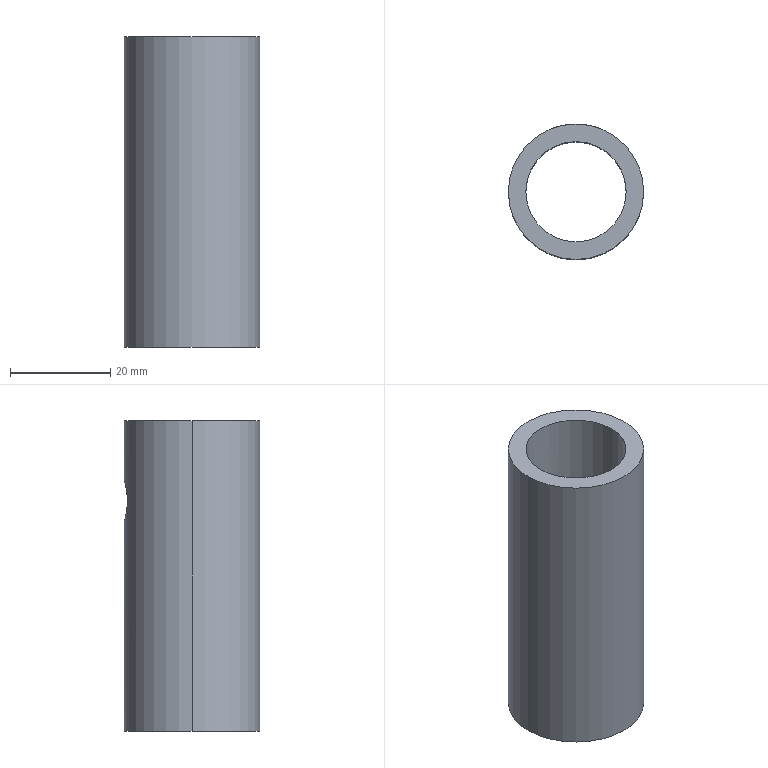Part | SolidWorks | features Extrusion 1, ICE 1 | 1 solid | 8 faces | box 27 x 27 x 62 mm | volume 15842 mm3 | cylinder 6 | plane 2 | commonest cylinder face diameters 8 x2 20 x2 27 x2
STEP:
#1=CARTESIAN_POINT('',(0.,13.5,-12.));
#2=VERTEX_POINT('',#1);
#3=CARTESIAN_POINT('',(0.,13.5,-20.));
#4=VERTEX_POINT('',#3);
#5=CARTESIAN_POINT('',(0.,13.5,-12.));
#6=CARTESIAN_POINT('',(-0.2619,13.5,-12.));
#7=CARTESIAN_POINT('',(-0.5246,13.492,-12.026));
#8=CARTESIAN_POINT('',(-1.044,13.462,-12.13));
#9=CARTESIAN_POINT('',(-1.294,13.44,-12.206));
#10=CARTESIAN_POINT('',(-1.776,13.385,-12.406));
#11=CARTESIAN_POINT('',(-2.01,13.351,-12.532));
#12=CARTESIAN_POINT('',(-2.443,13.279,-12.822));
#13=CARTESIAN_POINT('',(-2.643,13.24,-12.987));
#14=CARTESIAN_POINT('',(-3.013,13.161,-13.356));
#15=CARTESIAN_POINT('',(-3.18,13.121,-13.559));
#16=CARTESIAN_POINT('',(-3.468,13.048,-13.99));
#17=CARTESIAN_POINT('',(-3.592,13.014,-14.22));
#18=CARTESIAN_POINT('',(-3.795,12.956,-14.708));
#19=CARTESIAN_POINT('',(-3.871,12.933,-14.958));
#20=CARTESIAN_POINT('',(-3.973,12.902,-15.47));
#21=CARTESIAN_POINT('',(-4.,12.894,-15.736));
#22=CARTESIAN_POINT('',(-4.,12.894,-16.263));
#23=CARTESIAN_POINT('',(-3.974,12.902,-16.524));
#24=CARTESIAN_POINT('',(-3.872,12.933,-17.039));
#25=CARTESIAN_POINT('',(-3.794,12.956,-17.294));
#26=CARTESIAN_POINT('',(-3.594,13.013,-17.776));
#27=CARTESIAN_POINT('',(-3.471,13.047,-18.006));
#28=CARTESIAN_POINT('',(-3.178,13.121,-18.443));
#29=CARTESIAN_POINT('',(-3.013,13.161,-18.644));
#30=CARTESIAN_POINT('',(-2.646,13.239,-19.011));
#31=CARTESIAN_POINT('',(-2.442,13.279,-19.178));
#32=CARTESIAN_POINT('',(-2.009,13.352,-19.469));
#33=CARTESIAN_POINT('',(-1.78,13.384,-19.592));
#34=CARTESIAN_POINT('',(-1.297,13.44,-19.793));
#35=CARTESIAN_POINT('',(-1.042,13.462,-19.871));
#36=CARTESIAN_POINT('',(-0.5274,13.492,-19.974));
#37=CARTESIAN_POINT('',(-0.2658,13.5,-20.));
#38=CARTESIAN_POINT('',(0.,13.5,-20.));
#39=B_SPLINE_CURVE_WITH_KNOTS('',3,(#5,#6,#7,#8,#9,#10,#11,#12,#13,#14,#15,#16,#17,#18,#19,#20,#21,#22,#23,#24,#25,#26,#27,#28,#29,#30,#31,#32,#33,#34,#35,#36,#37,#38),.UNSPECIFIED.,.F.,.F.,(4,2,2,2,2,2,2,2,2,2,2,2,2,2,2,2,4),(0.01258,0.01336,0.01415,0.01493,0.01572,0.01651,0.01729,0.01808,0.01886,0.01965,0.02044,0.02122,0.02201,0.02279,0.02358,0.02436,0.02515),.UNSPECIFIED.);
#40=EDGE_CURVE('',#2,#4,#39,.T.);
#41=ORIENTED_EDGE('',*,*,#40,.F.);
#42=CARTESIAN_POINT('',(0.,10.,-12.));
#43=VERTEX_POINT('',#42);
#44=CARTESIAN_POINT('',(0.,62.,-12.));
#45=DIRECTION('',(0.,-1.,0.));
#46=VECTOR('',#45,1000.);
#47=LINE('',#44,#46);
#48=EDGE_CURVE('',#2,#43,#47,.T.);
#49=ORIENTED_EDGE('',*,*,#48,.T.);
#50=CARTESIAN_POINT('',(0.,10.,-20.));
#51=VERTEX_POINT('',#50);
#52=CARTESIAN_POINT('',(0.,10.,-12.));
#53=CARTESIAN_POINT('',(-0.2631,10.,-12.));
#54=CARTESIAN_POINT('',(-0.5298,9.989,-12.026));
#55=CARTESIAN_POINT('',(-1.048,9.948,-12.131));
#56=CARTESIAN_POINT('',(-1.299,9.918,-12.208));
#57=CARTESIAN_POINT('',(-1.782,9.843,-12.409));
#58=CARTESIAN_POINT('',(-2.015,9.797,-12.535));
#59=CARTESIAN_POINT('',(-2.446,9.699,-12.824));
#60=CARTESIAN_POINT('',(-2.646,9.645,-12.989));
#61=CARTESIAN_POINT('',(-3.015,9.537,-13.358));
#62=CARTESIAN_POINT('',(-3.179,9.483,-13.558));
#63=CARTESIAN_POINT('',(-3.466,9.381,-13.987));
#64=CARTESIAN_POINT('',(-3.592,9.333,-14.22));
#65=CARTESIAN_POINT('',(-3.793,9.253,-14.703));
#66=CARTESIAN_POINT('',(-3.869,9.221,-14.952));
#67=CARTESIAN_POINT('',(-3.973,9.177,-15.468));
#68=CARTESIAN_POINT('',(-4.,9.165,-15.736));
#69=CARTESIAN_POINT('',(-4.,9.165,-16.263));
#70=CARTESIAN_POINT('',(-3.974,9.177,-16.525));
#71=CARTESIAN_POINT('',(-3.87,9.221,-17.046));
#72=CARTESIAN_POINT('',(-3.792,9.254,-17.298));
#73=CARTESIAN_POINT('',(-3.592,9.333,-17.78));
#74=CARTESIAN_POINT('',(-3.467,9.381,-18.013));
#75=CARTESIAN_POINT('',(-3.177,9.483,-18.444));
#76=CARTESIAN_POINT('',(-3.013,9.537,-18.644));
#77=CARTESIAN_POINT('',(-2.646,9.645,-19.011));
#78=CARTESIAN_POINT('',(-2.443,9.699,-19.178));
#79=CARTESIAN_POINT('',(-2.014,9.798,-19.466));
#80=CARTESIAN_POINT('',(-1.785,9.842,-19.589));
#81=CARTESIAN_POINT('',(-1.298,9.918,-19.793));
#82=CARTESIAN_POINT('',(-1.046,9.948,-19.87));
#83=CARTESIAN_POINT('',(-0.5323,9.989,-19.973));
#84=CARTESIAN_POINT('',(-0.2671,10.,-20.));
#85=CARTESIAN_POINT('',(0.,10.,-20.));
#86=B_SPLINE_CURVE_WITH_KNOTS('',3,(#52,#53,#54,#55,#56,#57,#58,#59,#60,#61,#62,#63,#64,#65,#66,#67,#68,#69,#70,#71,#72,#73,#74,#75,#76,#77,#78,#79,#80,#81,#82,#83,#84,#85),.UNSPECIFIED.,.F.,.F.,(4,2,2,2,2,2,2,2,2,2,2,2,2,2,2,2,4),(0.01264,0.01343,0.01422,0.01501,0.0158,0.01659,0.01738,0.01817,0.01896,0.01974,0.02053,0.02132,0.02211,0.0229,0.02369,0.02448,0.02527),.UNSPECIFIED.);
#87=EDGE_CURVE('',#43,#51,#86,.T.);
#88=ORIENTED_EDGE('',*,*,#87,.T.);
#89=CARTESIAN_POINT('',(0.,62.,-20.));
#90=DIRECTION('',(0.,-1.,0.));
#91=VECTOR('',#90,1000.);
#92=LINE('',#89,#91);
#93=EDGE_CURVE('',#4,#51,#92,.T.);
#94=ORIENTED_EDGE('',*,*,#93,.F.);
#95=EDGE_LOOP('',(#41,#49,#88,#94));
#96=FACE_OUTER_BOUND('',#95,.T.);
#97=CARTESIAN_POINT('',(0.,62.,-16.));
#98=DIRECTION('',(0.,-1.,0.));
#99=DIRECTION('',(0.,0.,-1.));
#100=AXIS2_PLACEMENT_3D('',#97,#98,#99);
#101=CYLINDRICAL_SURFACE('',#100,4.);
#102=ADVANCED_FACE('',(#96),#101,.F.);
#103=CARTESIAN_POINT('',(-10.,0.,-62.));
#104=VERTEX_POINT('',#103);
#105=CARTESIAN_POINT('',(10.,0.,-62.));
#106=VERTEX_POINT('',#105);
#107=CARTESIAN_POINT('',(0.,0.,-62.));
#108=DIRECTION('',(0.,0.,1.));
#109=DIRECTION('',(1.,0.,0.));
#110=AXIS2_PLACEMENT_3D('',#107,#108,#109);
#111=CIRCLE('',#110,10.);
#112=EDGE_CURVE('',#104,#106,#111,.T.);
#113=ORIENTED_EDGE('',*,*,#112,.F.);
#114=CARTESIAN_POINT('',(-10.,0.,0.));
#115=VERTEX_POINT('',#114);
#116=CARTESIAN_POINT('',(-10.,0.,-62.));
#117=DIRECTION('',(0.,0.,1.));
#118=VECTOR('',#117,1000.);
#119=LINE('',#116,#118);
#120=EDGE_CURVE('',#104,#115,#119,.T.);
#121=ORIENTED_EDGE('',*,*,#120,.T.);
#122=CARTESIAN_POINT('',(10.,0.,0.));
#123=VERTEX_POINT('',#122);
#124=CARTESIAN_POINT('',(0.,0.,0.));
#125=DIRECTION('',(0.,0.,1.));
#126=DIRECTION('',(1.,0.,0.));
#127=AXIS2_PLACEMENT_3D('',#124,#125,#126);
#128=CIRCLE('',#127,10.);
#129=EDGE_CURVE('',#115,#123,#128,.T.);
#130=ORIENTED_EDGE('',*,*,#129,.T.);
#131=CARTESIAN_POINT('',(10.,0.,-62.));
#132=DIRECTION('',(0.,0.,1.));
#133=VECTOR('',#132,1000.);
#134=LINE('',#131,#133);
#135=EDGE_CURVE('',#106,#123,#134,.T.);
#136=ORIENTED_EDGE('',*,*,#135,.F.);
#137=EDGE_LOOP('',(#113,#121,#130,#136));
#138=FACE_OUTER_BOUND('',#137,.T.);
#139=CARTESIAN_POINT('',(0.,0.,-62.));
#140=DIRECTION('',(0.,0.,1.));
#141=DIRECTION('',(1.,0.,0.));
#142=AXIS2_PLACEMENT_3D('',#139,#140,#141);
#143=CYLINDRICAL_SURFACE('',#142,10.);
#144=ADVANCED_FACE('',(#138),#143,.F.);
#145=CARTESIAN_POINT('',(0.,13.5,-20.));
#146=CARTESIAN_POINT('',(0.2659,13.5,-20.));
#147=CARTESIAN_POINT('',(0.5271,13.492,-19.974));
#148=CARTESIAN_POINT('',(1.04,13.462,-19.871));
#149=CARTESIAN_POINT('',(1.295,13.44,-19.794));
#150=CARTESIAN_POINT('',(1.779,13.384,-19.592));
#151=CARTESIAN_POINT('',(2.008,13.352,-19.469));
#152=CARTESIAN_POINT('',(2.442,13.279,-19.179));
#153=CARTESIAN_POINT('',(2.646,13.239,-19.011));
#154=CARTESIAN_POINT('',(3.013,13.161,-18.644));
#155=CARTESIAN_POINT('',(3.178,13.122,-18.443));
#156=CARTESIAN_POINT('',(3.47,13.047,-18.007));
#157=CARTESIAN_POINT('',(3.593,13.013,-17.776));
#158=CARTESIAN_POINT('',(3.793,12.957,-17.296));
#159=CARTESIAN_POINT('',(3.871,12.933,-17.042));
#160=CARTESIAN_POINT('',(3.974,12.902,-16.525));
#161=CARTESIAN_POINT('',(4.,12.894,-16.264));
#162=CARTESIAN_POINT('',(4.,12.894,-15.739));
#163=CARTESIAN_POINT('',(3.974,12.902,-15.472));
#164=CARTESIAN_POINT('',(3.871,12.933,-14.958));
#165=CARTESIAN_POINT('',(3.795,12.956,-14.708));
#166=CARTESIAN_POINT('',(3.593,13.014,-14.222));
#167=CARTESIAN_POINT('',(3.468,13.048,-13.99));
#168=CARTESIAN_POINT('',(3.179,13.121,-13.559));
#169=CARTESIAN_POINT('',(3.012,13.161,-13.355));
#170=CARTESIAN_POINT('',(2.643,13.24,-12.986));
#171=CARTESIAN_POINT('',(2.442,13.279,-12.822));
#172=CARTESIAN_POINT('',(2.01,13.351,-12.532));
#173=CARTESIAN_POINT('',(1.776,13.385,-12.406));
#174=CARTESIAN_POINT('',(1.294,13.44,-12.206));
#175=CARTESIAN_POINT('',(1.044,13.462,-12.13));
#176=CARTESIAN_POINT('',(0.5275,13.492,-12.026));
#177=CARTESIAN_POINT('',(0.262,13.5,-12.));
#178=CARTESIAN_POINT('',(0.,13.5,-12.));
#179=B_SPLINE_CURVE_WITH_KNOTS('',3,(#145,#146,#147,#148,#149,#150,#151,#152,#153,#154,#155,#156,#157,#158,#159,#160,#161,#162,#163,#164,#165,#166,#167,#168,#169,#170,#171,#172,#173,#174,#175,#176,#177,#178),.UNSPECIFIED.,.F.,.F.,(4,2,2,2,2,2,2,2,2,2,2,2,2,2,2,2,4),(0.,0.0007861,0.001572,0.002358,0.003144,0.00393,0.004716,0.005502,0.006288,0.007074,0.007861,0.008647,0.009433,0.01022,0.011,0.01179,0.01258),.UNSPECIFIED.);
#180=EDGE_CURVE('',#4,#2,#179,.T.);
#181=ORIENTED_EDGE('',*,*,#180,.T.);
#182=ORIENTED_EDGE('',*,*,#40,.T.);
#183=EDGE_LOOP('',(#181,#182));
#184=FACE_BOUND('',#183,.T.);
#185=CARTESIAN_POINT('',(13.5,0.,-62.));
#186=VERTEX_POINT('',#185);
#187=CARTESIAN_POINT('',(-13.5,0.,-62.));
#188=VERTEX_POINT('',#187);
#189=CARTESIAN_POINT('',(0.,0.,-62.));
#190=DIRECTION('',(0.,0.,1.));
#191=DIRECTION('',(1.,0.,0.));
#192=AXIS2_PLACEMENT_3D('',#189,#190,#191);
#193=CIRCLE('',#192,13.5);
#194=EDGE_CURVE('',#186,#188,#193,.T.);
#195=ORIENTED_EDGE('',*,*,#194,.T.);
#196=CARTESIAN_POINT('',(-13.5,0.,0.));
#197=VERTEX_POINT('',#196);
#198=CARTESIAN_POINT('',(-13.5,0.,-62.));
#199=DIRECTION('',(0.,0.,1.));
#200=VECTOR('',#199,1000.);
#201=LINE('',#198,#200);
#202=EDGE_CURVE('',#188,#197,#201,.T.);
#203=ORIENTED_EDGE('',*,*,#202,.T.);
#204=CARTESIAN_POINT('',(13.5,0.,0.));
#205=VERTEX_POINT('',#204);
#206=CARTESIAN_POINT('',(0.,0.,0.));
#207=DIRECTION('',(0.,0.,1.));
#208=DIRECTION('',(1.,0.,0.));
#209=AXIS2_PLACEMENT_3D('',#206,#207,#208);
#210=CIRCLE('',#209,13.5);
#211=EDGE_CURVE('',#205,#197,#210,.T.);
#212=ORIENTED_EDGE('',*,*,#211,.F.);
#213=CARTESIAN_POINT('',(13.5,0.,-62.));
#214=DIRECTION('',(0.,0.,1.));
#215=VECTOR('',#214,1000.);
#216=LINE('',#213,#215);
#217=EDGE_CURVE('',#186,#205,#216,.T.);
#218=ORIENTED_EDGE('',*,*,#217,.F.);
#219=EDGE_LOOP('',(#195,#203,#212,#218));
#220=FACE_OUTER_BOUND('',#219,.T.);
#221=CARTESIAN_POINT('',(0.,0.,-62.));
#222=DIRECTION('',(0.,0.,1.));
#223=DIRECTION('',(1.,0.,0.));
#224=AXIS2_PLACEMENT_3D('',#221,#222,#223);
#225=CYLINDRICAL_SURFACE('',#224,13.5);
#226=ADVANCED_FACE('',(#184,#220),#225,.T.);
#227=ORIENTED_EDGE('',*,*,#202,.F.);
#228=CARTESIAN_POINT('',(0.,0.,-62.));
#229=DIRECTION('',(0.,0.,1.));
#230=DIRECTION('',(1.,0.,0.));
#231=AXIS2_PLACEMENT_3D('',#228,#229,#230);
#232=CIRCLE('',#231,13.5);
#233=EDGE_CURVE('',#188,#186,#232,.T.);
#234=ORIENTED_EDGE('',*,*,#233,.T.);
#235=ORIENTED_EDGE('',*,*,#217,.T.);
#236=CARTESIAN_POINT('',(0.,0.,0.));
#237=DIRECTION('',(0.,0.,1.));
#238=DIRECTION('',(1.,0.,0.));
#239=AXIS2_PLACEMENT_3D('',#236,#237,#238);
#240=CIRCLE('',#239,13.5);
#241=EDGE_CURVE('',#197,#205,#240,.T.);
#242=ORIENTED_EDGE('',*,*,#241,.F.);
#243=EDGE_LOOP('',(#227,#234,#235,#242));
#244=FACE_OUTER_BOUND('',#243,.T.);
#245=CARTESIAN_POINT('',(0.,0.,-62.));
#246=DIRECTION('',(0.,0.,1.));
#247=DIRECTION('',(1.,0.,0.));
#248=AXIS2_PLACEMENT_3D('',#245,#246,#247);
#249=CYLINDRICAL_SURFACE('',#248,13.5);
#250=ADVANCED_FACE('',(#244),#249,.T.);
#251=ORIENTED_EDGE('',*,*,#120,.F.);
#252=CARTESIAN_POINT('',(0.,0.,-62.));
#253=DIRECTION('',(0.,0.,1.));
#254=DIRECTION('',(1.,0.,0.));
#255=AXIS2_PLACEMENT_3D('',#252,#253,#254);
#256=CIRCLE('',#255,10.);
#257=EDGE_CURVE('',#106,#104,#256,.T.);
#258=ORIENTED_EDGE('',*,*,#257,.F.);
#259=ORIENTED_EDGE('',*,*,#135,.T.);
#260=CARTESIAN_POINT('',(0.,0.,0.));
#261=DIRECTION('',(0.,0.,1.));
#262=DIRECTION('',(1.,0.,0.));
#263=AXIS2_PLACEMENT_3D('',#260,#261,#262);
#264=CIRCLE('',#263,10.);
#265=EDGE_CURVE('',#123,#115,#264,.T.);
#266=ORIENTED_EDGE('',*,*,#265,.T.);
#267=EDGE_LOOP('',(#251,#258,#259,#266));
#268=FACE_OUTER_BOUND('',#267,.T.);
#269=CARTESIAN_POINT('',(0.,10.,-20.));
#270=CARTESIAN_POINT('',(0.2673,10.,-20.));
#271=CARTESIAN_POINT('',(0.5296,9.989,-19.973));
#272=CARTESIAN_POINT('',(1.045,9.949,-19.87));
#273=CARTESIAN_POINT('',(1.3,9.918,-19.792));
#274=CARTESIAN_POINT('',(1.784,9.843,-19.59));
#275=CARTESIAN_POINT('',(2.013,9.798,-19.467));
#276=CARTESIAN_POINT('',(2.445,9.699,-19.176));
#277=CARTESIAN_POINT('',(2.648,9.645,-19.009));
#278=CARTESIAN_POINT('',(3.013,9.537,-18.644));
#279=CARTESIAN_POINT('',(3.178,9.483,-18.444));
#280=CARTESIAN_POINT('',(3.469,9.38,-18.009));
#281=CARTESIAN_POINT('',(3.591,9.333,-17.78));
#282=CARTESIAN_POINT('',(3.792,9.254,-17.3));
#283=CARTESIAN_POINT('',(3.87,9.221,-17.046));
#284=CARTESIAN_POINT('',(3.974,9.177,-16.528));
#285=CARTESIAN_POINT('',(4.,9.165,-16.267));
#286=CARTESIAN_POINT('',(4.,9.165,-15.738));
#287=CARTESIAN_POINT('',(3.973,9.177,-15.47));
#288=CARTESIAN_POINT('',(3.87,9.221,-14.955));
#289=CARTESIAN_POINT('',(3.793,9.253,-14.703));
#290=CARTESIAN_POINT('',(3.59,9.334,-14.216));
#291=CARTESIAN_POINT('',(3.466,9.381,-13.987));
#292=CARTESIAN_POINT('',(3.178,9.483,-13.557));
#293=CARTESIAN_POINT('',(3.01,9.538,-13.354));
#294=CARTESIAN_POINT('',(2.644,9.646,-12.988));
#295=CARTESIAN_POINT('',(2.445,9.699,-12.824));
#296=CARTESIAN_POINT('',(2.013,9.798,-12.534));
#297=CARTESIAN_POINT('',(1.78,9.843,-12.408));
#298=CARTESIAN_POINT('',(1.299,9.918,-12.208));
#299=CARTESIAN_POINT('',(1.049,9.948,-12.131));
#300=CARTESIAN_POINT('',(0.5273,9.99,-12.026));
#301=CARTESIAN_POINT('',(0.2633,10.,-12.));
#302=CARTESIAN_POINT('',(0.,10.,-12.));
#303=B_SPLINE_CURVE_WITH_KNOTS('',3,(#269,#270,#271,#272,#273,#274,#275,#276,#277,#278,#279,#280,#281,#282,#283,#284,#285,#286,#287,#288,#289,#290,#291,#292,#293,#294,#295,#296,#297,#298,#299,#300,#301,#302),.UNSPECIFIED.,.F.,.F.,(4,2,2,2,2,2,2,2,2,2,2,2,2,2,2,2,4),(0.,0.00079,0.00158,0.00237,0.00316,0.00395,0.00474,0.00553,0.00632,0.00711,0.0079,0.00869,0.00948,0.01027,0.01106,0.01185,0.01264),.UNSPECIFIED.);
#304=EDGE_CURVE('',#51,#43,#303,.T.);
#305=ORIENTED_EDGE('',*,*,#304,.F.);
#306=ORIENTED_EDGE('',*,*,#87,.F.);
#307=EDGE_LOOP('',(#305,#306));
#308=FACE_BOUND('',#307,.T.);
#309=CARTESIAN_POINT('',(0.,0.,-62.));
#310=DIRECTION('',(0.,0.,1.));
#311=DIRECTION('',(1.,0.,0.));
#312=AXIS2_PLACEMENT_3D('',#309,#310,#311);
#313=CYLINDRICAL_SURFACE('',#312,10.);
#314=ADVANCED_FACE('',(#268,#308),#313,.F.);
#315=ORIENTED_EDGE('',*,*,#257,.T.);
#316=ORIENTED_EDGE('',*,*,#112,.T.);
#317=EDGE_LOOP('',(#315,#316));
#318=FACE_BOUND('',#317,.T.);
#319=ORIENTED_EDGE('',*,*,#194,.F.);
#320=ORIENTED_EDGE('',*,*,#233,.F.);
#321=EDGE_LOOP('',(#319,#320));
#322=FACE_OUTER_BOUND('',#321,.T.);
#323=CARTESIAN_POINT('',(0.,0.,-62.));
#324=DIRECTION('',(0.,0.,1.));
#325=DIRECTION('',(1.,0.,0.));
#326=AXIS2_PLACEMENT_3D('',#323,#324,#325);
#327=PLANE('',#326);
#328=ADVANCED_FACE('',(#318,#322),#327,.F.);
#329=ORIENTED_EDGE('',*,*,#265,.F.);
#330=ORIENTED_EDGE('',*,*,#129,.F.);
#331=EDGE_LOOP('',(#329,#330));
#332=FACE_BOUND('',#331,.T.);
#333=ORIENTED_EDGE('',*,*,#211,.T.);
#334=ORIENTED_EDGE('',*,*,#241,.T.);
#335=EDGE_LOOP('',(#333,#334));
#336=FACE_OUTER_BOUND('',#335,.T.);
#337=CARTESIAN_POINT('',(0.,0.,0.));
#338=DIRECTION('',(0.,0.,1.));
#339=DIRECTION('',(1.,0.,0.));
#340=AXIS2_PLACEMENT_3D('',#337,#338,#339);
#341=PLANE('',#340);
#342=ADVANCED_FACE('',(#332,#336),#341,.T.);
#343=ORIENTED_EDGE('',*,*,#48,.F.);
#344=ORIENTED_EDGE('',*,*,#180,.F.);
#345=ORIENTED_EDGE('',*,*,#93,.T.);
#346=ORIENTED_EDGE('',*,*,#304,.T.);
#347=EDGE_LOOP('',(#343,#344,#345,#346));
#348=FACE_OUTER_BOUND('',#347,.T.);
#349=CARTESIAN_POINT('',(0.,62.,-16.));
#350=DIRECTION('',(0.,-1.,0.));
#351=DIRECTION('',(0.,0.,-1.));
#352=AXIS2_PLACEMENT_3D('',#349,#350,#351);
#353=CYLINDRICAL_SURFACE('',#352,4.);
#354=ADVANCED_FACE('',(#348),#353,.F.);
#355=CLOSED_SHELL('',(#102,#144,#226,#250,#314,#328,#342,#354));
#356=MANIFOLD_SOLID_BREP('',#355);
#357=CARTESIAN_POINT('',(0.,0.,0.));
#358=DIRECTION('',(0.,0.,1.));
#359=DIRECTION('',(1.,0.,0.));
#360=AXIS2_PLACEMENT_3D('',#357,#358,#359);
#361=(LENGTH_UNIT()NAMED_UNIT(*)SI_UNIT(.MILLI.,.METRE.));
#362=UNCERTAINTY_MEASURE_WITH_UNIT(LENGTH_MEASURE(0.00001),#361,'','');
#363=(NAMED_UNIT(*)PLANE_ANGLE_UNIT()SI_UNIT($,.RADIAN.));
#364=(NAMED_UNIT(*)SI_UNIT($,.STERADIAN.)SOLID_ANGLE_UNIT());
#365=(GEOMETRIC_REPRESENTATION_CONTEXT(3)GLOBAL_UNCERTAINTY_ASSIGNED_CONTEXT((#362))GLOBAL_UNIT_ASSIGNED_CONTEXT((#361,#363,#364))REPRESENTATION_CONTEXT('',''));
#366=ADVANCED_BREP_SHAPE_REPRESENTATION('',(#356,#360),#365);